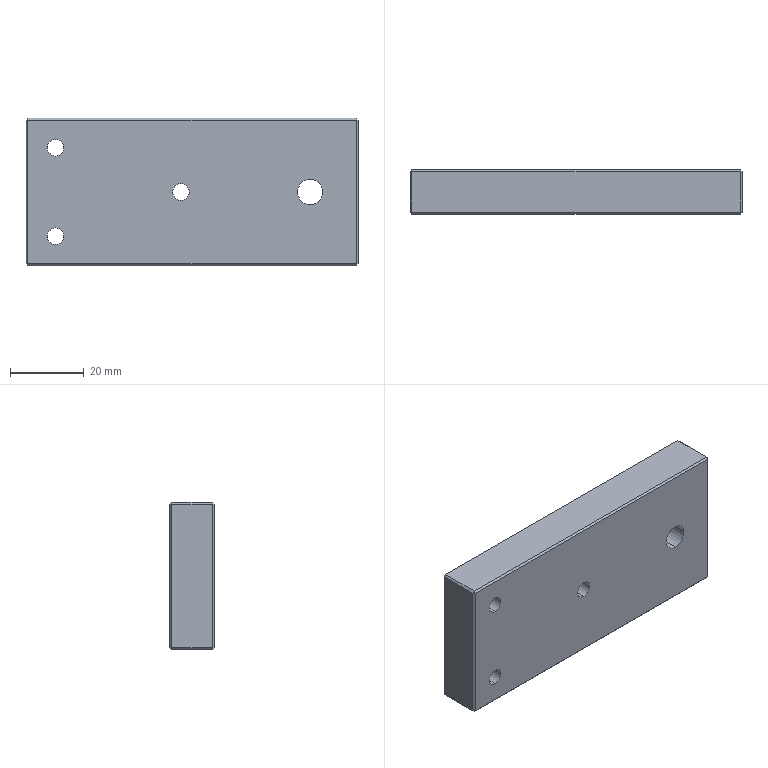Part | STEP file | ND25021-01-JDKM-29-TL | 1 solid | 43 faces | box 90 x 12 x 40 mm | volume 41668 mm3 | plane 29 | cylinder 14 | commonest cylinder face diameters 4.5 x6 8 x6 6.8 x2